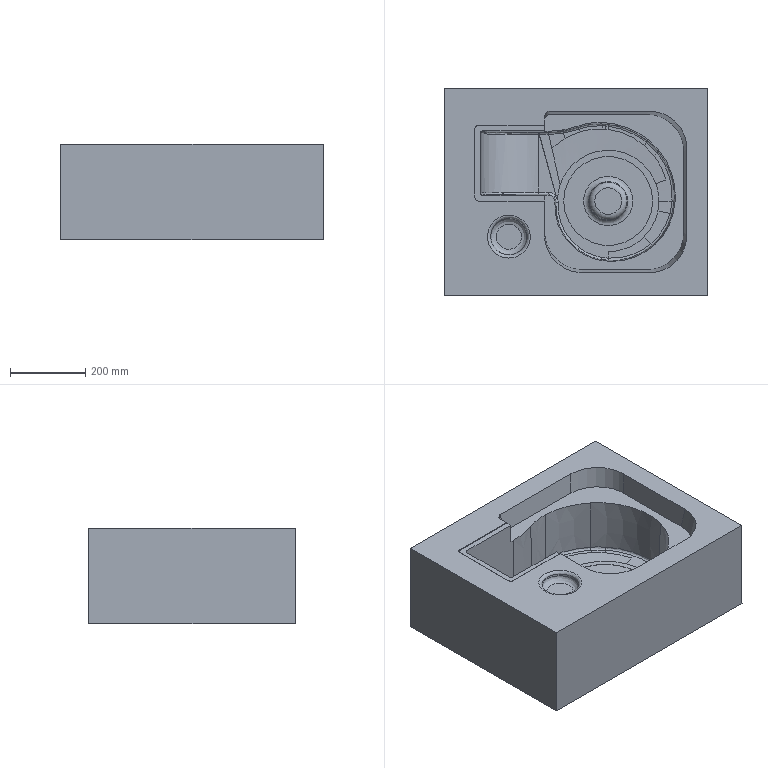NC program | NX | posted with a generic post | part box 700 x 550 x 255 mm
Lines 30859 to 30947 of 43405:
(FACE_MILLING_1 , TOOL : D26R0.8)
N61692 M6
N61694 G54
N61696 G17 G0 G90 X85.723 Y-85.502 S0 M3
N61698 G43 Z30. H0
N61700 Z-176.05
N61702 G94 G1 Z-179.05 F250.
N61704 Y-72.402
N61706 G2 X37.248 Y-23.927 R48.475
N61708 X85.723 Y-72.402 R-48.475
N61710 G1 Y-59.402
N61712 G2 X50.248 Y-23.927 R35.475
N61714 X85.723 Y-59.402 R-35.475
N61716 G1 Y-46.402
N61718 G2 X63.248 Y-23.927 R22.475
N61720 X85.723 Y-46.402 R-22.475
N61722 G1 Y-33.402
N61724 G2 X76.248 Y-23.927 R9.475
N61726 X85.723 Y-33.402 R-9.475
N61728 G1 Y-46.402
N61730 Z-176.05
N61732 G0 Z30.
N61734 X-40.391 Y46.518
N61736 Z-201.05
N61738 G1 Z-204.05
N61740 X-27.764 Y42.215
N61742 G2 X-26.881 Y41.905 R52.
N61744 X10.673 Y-130.609 R-130.436
N61746 X9.998 Y-131.258 R52.
N61748 G1 Z-201.05
N61750 G0 Z30.
N61752 X-46.552 Y34.129
N61754 Z-201.05
N61756 G1 Z-204.05
N61758 X-33.828 Y30.495
N61760 G2 X-21.334 Y24.341 R39.
N61762 X8.416 Y-112.329 R-117.436
N61764 X-0.388 Y-123.119 R39.
N61766 G1 Z-201.05
N61768 G0 Z30.
N61770 X-51.47 Y21.298
N61772 Z-201.05
N61774 G1 Z-204.05
N61776 X-38.653 Y18.32
N61778 G2 X-22.953 Y7.489 R26.
N61780 X-16.936 Y-3.919 R60.964
N61782 G1 X-16.83 Y-4.185
N61784 G2 X-5.629 Y-74.54 R-104.436
N61786 G3 X-2.317 Y-82.131 R104.671
N61788 G2 X-9.838 Y-114.051 R26.
N61790 G1 Z-201.05
N61792 G0 Z30.
N61794 X-52.845 Y16.893
N61796 Z-201.05
N61798 G1 Z-204.05
N61800 X-55.02 Y8.098
N61802 X-42.227 Y5.787
N61804 G2 X-33.745 Y0.242 R13.
N61806 X-29.007 Y-8.745 R47.964
N61808 X-25.585 Y-29.702 R48.717
N61810 G3 X-14.017 Y-87.797 R117.671
N61812 G2 X-18.298 Y-104.138 R13.
N61814 G1 Z-201.05
N61816 G0 Z30.
N61818 X-63.028 Y20.53
N61820 Z-201.05
N61822 G1 Z-204.05
N61824 X-44.538 Y-7.006
N61826 G2 X-41.078 Y-13.571 R34.964
N61828 X-38.564 Y-28.95 R35.717
N61830 G3 X-25.717 Y-93.463 R130.671
N61832 G1 X-18.835 Y-104.492
N61834 Z-201.05
N61836 G0 Z30.
N61838 X190.158 Y-23.927
N61840 Z-201.05
N61842 G1 Z-204.05
N61844 X177.158
N61846 G2 X85.723 Y-115.363 R91.436
N61848 X177.158 Y-23.927 R-91.436
N61850 G1 X164.158
N61852 G2 X85.723 Y-102.363 R78.436
N61854 X164.158 Y-23.927 R-78.436
N61856 G1 X177.158
N61858 Z-201.05
N61860 G0 Z30.
N61862 M5